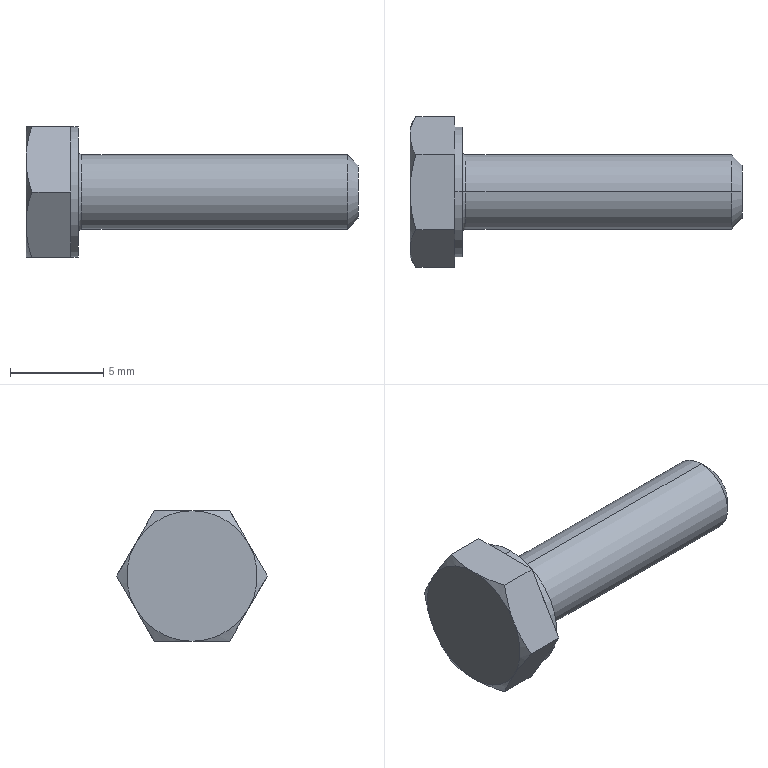Part | SolidWorks | features RevCut 4, Chamfer 1, Extrusion 1, Fillet 1, LPattern 1, Revolution 1 | 1 solid | 29 faces | box 17.8 x 8.083 x 7 mm | volume 303.684 mm3 | plane 15 | cone 8 | cylinder 4 | torus 2 | commonest cylinder face diameters 4 x2 7 x2
STEP:
#1=CARTESIAN_POINT('',(3.,0.,2.));
#2=VERTEX_POINT('',#1);
#3=CARTESIAN_POINT('',(3.,0.,-2.));
#4=VERTEX_POINT('',#3);
#5=CARTESIAN_POINT('',(3.,0.,0.));
#6=DIRECTION('',(1.,0.,0.));
#7=DIRECTION('',(0.,0.,-1.));
#8=AXIS2_PLACEMENT_3D('',#5,#6,#7);
#9=CIRCLE('',#8,2.);
#10=EDGE_CURVE('',#2,#4,#9,.T.);
#11=ORIENTED_EDGE('',*,*,#10,.F.);
#12=CARTESIAN_POINT('',(2.8,0.,2.2));
#13=VERTEX_POINT('',#12);
#14=CARTESIAN_POINT('',(3.,0.,2.2));
#15=DIRECTION('',(0.,1.,0.));
#16=DIRECTION('',(0.,0.,1.));
#17=AXIS2_PLACEMENT_3D('',#14,#15,#16);
#18=CIRCLE('',#17,0.2);
#19=EDGE_CURVE('',#2,#13,#18,.T.);
#20=ORIENTED_EDGE('',*,*,#19,.T.);
#21=CARTESIAN_POINT('',(2.8,0.,-2.2));
#22=VERTEX_POINT('',#21);
#23=CARTESIAN_POINT('',(2.8,0.,0.));
#24=DIRECTION('',(-1.,0.,0.));
#25=DIRECTION('',(0.,0.,-1.));
#26=AXIS2_PLACEMENT_3D('',#23,#24,#25);
#27=CIRCLE('',#26,2.2);
#28=EDGE_CURVE('',#22,#13,#27,.T.);
#29=ORIENTED_EDGE('',*,*,#28,.F.);
#30=CARTESIAN_POINT('',(3.,0.,-2.2));
#31=DIRECTION('',(0.,-1.,0.));
#32=DIRECTION('',(0.,0.,-1.));
#33=AXIS2_PLACEMENT_3D('',#30,#31,#32);
#34=CIRCLE('',#33,0.2);
#35=EDGE_CURVE('',#4,#22,#34,.T.);
#36=ORIENTED_EDGE('',*,*,#35,.F.);
#37=EDGE_LOOP('',(#11,#20,#29,#36));
#38=FACE_OUTER_BOUND('',#37,.T.);
#39=CARTESIAN_POINT('',(3.,0.,0.));
#40=DIRECTION('',(1.,0.,0.));
#41=DIRECTION('',(0.,0.,-1.));
#42=AXIS2_PLACEMENT_3D('',#39,#40,#41);
#43=TOROIDAL_SURFACE('',#42,2.2,0.2);
#44=ADVANCED_FACE('',(#38),#43,.F.);
#45=CARTESIAN_POINT('',(17.8,0.,-1.44));
#46=VERTEX_POINT('',#45);
#47=CARTESIAN_POINT('',(17.8,0.,1.44));
#48=VERTEX_POINT('',#47);
#49=CARTESIAN_POINT('',(17.8,0.,0.));
#50=DIRECTION('',(1.,0.,0.));
#51=DIRECTION('',(0.,0.,1.));
#52=AXIS2_PLACEMENT_3D('',#49,#50,#51);
#53=CIRCLE('',#52,1.44);
#54=EDGE_CURVE('',#46,#48,#53,.T.);
#55=ORIENTED_EDGE('',*,*,#54,.F.);
#56=CARTESIAN_POINT('',(17.24,0.,-2.));
#57=VERTEX_POINT('',#56);
#58=CARTESIAN_POINT('',(17.24,0.,-2.));
#59=DIRECTION('',(-0.7071,0.,-0.7071));
#60=VECTOR('',#59,1000.);
#61=LINE('',#58,#60);
#62=EDGE_CURVE('',#46,#57,#61,.T.);
#63=ORIENTED_EDGE('',*,*,#62,.T.);
#64=CARTESIAN_POINT('',(17.24,0.,2.));
#65=VERTEX_POINT('',#64);
#66=CARTESIAN_POINT('',(17.24,0.,0.));
#67=DIRECTION('',(-1.,0.,0.));
#68=DIRECTION('',(0.,0.,1.));
#69=AXIS2_PLACEMENT_3D('',#66,#67,#68);
#70=CIRCLE('',#69,2.);
#71=EDGE_CURVE('',#65,#57,#70,.T.);
#72=ORIENTED_EDGE('',*,*,#71,.F.);
#73=CARTESIAN_POINT('',(17.24,0.,2.));
#74=DIRECTION('',(-0.7071,0.,0.7071));
#75=VECTOR('',#74,1000.);
#76=LINE('',#73,#75);
#77=EDGE_CURVE('',#48,#65,#76,.T.);
#78=ORIENTED_EDGE('',*,*,#77,.F.);
#79=EDGE_LOOP('',(#55,#63,#72,#78));
#80=FACE_OUTER_BOUND('',#79,.T.);
#81=CARTESIAN_POINT('',(17.24,0.,0.));
#82=DIRECTION('',(-1.,0.,0.));
#83=DIRECTION('',(0.,0.,1.));
#84=AXIS2_PLACEMENT_3D('',#81,#82,#83);
#85=CONICAL_SURFACE('',#84,2.,0.7854);
#86=ADVANCED_FACE('',(#80),#85,.T.);
#87=ORIENTED_EDGE('',*,*,#71,.T.);
#88=CARTESIAN_POINT('',(0.,0.,-2.));
#89=DIRECTION('',(-1.,0.,0.));
#90=VECTOR('',#89,1000.);
#91=LINE('',#88,#90);
#92=EDGE_CURVE('',#57,#4,#91,.T.);
#93=ORIENTED_EDGE('',*,*,#92,.T.);
#94=CARTESIAN_POINT('',(3.,0.,0.));
#95=DIRECTION('',(1.,0.,0.));
#96=DIRECTION('',(0.,0.,-1.));
#97=AXIS2_PLACEMENT_3D('',#94,#95,#96);
#98=CIRCLE('',#97,2.);
#99=EDGE_CURVE('',#4,#2,#98,.T.);
#100=ORIENTED_EDGE('',*,*,#99,.T.);
#101=CARTESIAN_POINT('',(0.,0.,2.));
#102=DIRECTION('',(-1.,0.,0.));
#103=VECTOR('',#102,1000.);
#104=LINE('',#101,#103);
#105=EDGE_CURVE('',#65,#2,#104,.T.);
#106=ORIENTED_EDGE('',*,*,#105,.F.);
#107=EDGE_LOOP('',(#87,#93,#100,#106));
#108=FACE_OUTER_BOUND('',#107,.T.);
#109=CARTESIAN_POINT('',(0.,0.,0.));
#110=DIRECTION('',(-1.,0.,0.));
#111=DIRECTION('',(0.,0.,1.));
#112=AXIS2_PLACEMENT_3D('',#109,#110,#111);
#113=CYLINDRICAL_SURFACE('',#112,2.);
#114=ADVANCED_FACE('',(#108),#113,.T.);
#115=CARTESIAN_POINT('',(2.8,0.,-3.5));
#116=VERTEX_POINT('',#115);
#117=CARTESIAN_POINT('',(2.8,0.,3.5));
#118=VERTEX_POINT('',#117);
#119=CARTESIAN_POINT('',(2.8,0.,0.));
#120=DIRECTION('',(1.,0.,0.));
#121=DIRECTION('',(0.,0.,-1.));
#122=AXIS2_PLACEMENT_3D('',#119,#120,#121);
#123=CIRCLE('',#122,3.5);
#124=EDGE_CURVE('',#116,#118,#123,.T.);
#125=ORIENTED_EDGE('',*,*,#124,.F.);
#126=CARTESIAN_POINT('',(2.4,0.,-3.5));
#127=VERTEX_POINT('',#126);
#128=CARTESIAN_POINT('',(0.,0.,-3.5));
#129=DIRECTION('',(-1.,0.,0.));
#130=VECTOR('',#129,1000.);
#131=LINE('',#128,#130);
#132=EDGE_CURVE('',#116,#127,#131,.T.);
#133=ORIENTED_EDGE('',*,*,#132,.T.);
#134=CARTESIAN_POINT('',(2.4,3.031,-1.75));
#135=VERTEX_POINT('',#134);
#136=CARTESIAN_POINT('',(2.4,0.,0.));
#137=DIRECTION('',(-1.,0.,0.));
#138=DIRECTION('',(0.,0.,1.));
#139=AXIS2_PLACEMENT_3D('',#136,#137,#138);
#140=CIRCLE('',#139,3.5);
#141=EDGE_CURVE('',#135,#127,#140,.T.);
#142=ORIENTED_EDGE('',*,*,#141,.F.);
#143=CARTESIAN_POINT('',(2.4,3.031,1.75));
#144=VERTEX_POINT('',#143);
#145=CARTESIAN_POINT('',(2.4,0.,0.));
#146=DIRECTION('',(-1.,0.,0.));
#147=DIRECTION('',(0.,0.,1.));
#148=AXIS2_PLACEMENT_3D('',#145,#146,#147);
#149=CIRCLE('',#148,3.5);
#150=EDGE_CURVE('',#144,#135,#149,.T.);
#151=ORIENTED_EDGE('',*,*,#150,.F.);
#152=CARTESIAN_POINT('',(2.4,0.,3.5));
#153=VERTEX_POINT('',#152);
#154=CARTESIAN_POINT('',(2.4,0.,0.));
#155=DIRECTION('',(-1.,0.,0.));
#156=DIRECTION('',(0.,0.,1.));
#157=AXIS2_PLACEMENT_3D('',#154,#155,#156);
#158=CIRCLE('',#157,3.5);
#159=EDGE_CURVE('',#153,#144,#158,.T.);
#160=ORIENTED_EDGE('',*,*,#159,.F.);
#161=CARTESIAN_POINT('',(0.,0.,3.5));
#162=DIRECTION('',(-1.,0.,0.));
#163=VECTOR('',#162,1000.);
#164=LINE('',#161,#163);
#165=EDGE_CURVE('',#118,#153,#164,.T.);
#166=ORIENTED_EDGE('',*,*,#165,.F.);
#167=EDGE_LOOP('',(#125,#133,#142,#151,#160,#166));
#168=FACE_OUTER_BOUND('',#167,.T.);
#169=CARTESIAN_POINT('',(0.,0.,0.));
#170=DIRECTION('',(-1.,0.,0.));
#171=DIRECTION('',(0.,0.,1.));
#172=AXIS2_PLACEMENT_3D('',#169,#170,#171);
#173=CYLINDRICAL_SURFACE('',#172,3.5);
#174=ADVANCED_FACE('',(#168),#173,.T.);
#175=CARTESIAN_POINT('',(2.4,2.021,-3.5));
#176=VERTEX_POINT('',#175);
#177=CARTESIAN_POINT('',(2.4,2.021,-3.5));
#178=DIRECTION('',(0.,0.5,0.866));
#179=VECTOR('',#178,1000.);
#180=LINE('',#177,#179);
#181=EDGE_CURVE('',#176,#135,#180,.T.);
#182=ORIENTED_EDGE('',*,*,#181,.F.);
#183=CARTESIAN_POINT('',(0.3126,2.021,-3.5));
#184=VERTEX_POINT('',#183);
#185=CARTESIAN_POINT('',(2.8,2.021,-3.5));
#186=DIRECTION('',(-1.,0.,0.));
#187=VECTOR('',#186,1000.);
#188=LINE('',#185,#187);
#189=EDGE_CURVE('',#176,#184,#188,.T.);
#190=ORIENTED_EDGE('',*,*,#189,.T.);
#191=CARTESIAN_POINT('',(0.,3.031,-1.75));
#192=VERTEX_POINT('',#191);
#193=CARTESIAN_POINT('',(0.,3.031,-1.75));
#194=CARTESIAN_POINT('',(0.,2.86,-2.047));
#195=CARTESIAN_POINT('',(0.02993,2.688,-2.344));
#196=CARTESIAN_POINT('',(0.1388,2.352,-2.926));
#197=CARTESIAN_POINT('',(0.2174,2.186,-3.214));
#198=CARTESIAN_POINT('',(0.3126,2.021,-3.5));
#199=B_SPLINE_CURVE_WITH_KNOTS('',3,(#193,#194,#195,#196,#197,#198),.UNSPECIFIED.,.F.,.F.,(4,2,4),(0.002045,0.003063,0.004082),.UNSPECIFIED.);
#200=EDGE_CURVE('',#192,#184,#199,.T.);
#201=ORIENTED_EDGE('',*,*,#200,.F.);
#202=CARTESIAN_POINT('',(0.3126,4.041,0.));
#203=VERTEX_POINT('',#202);
#204=CARTESIAN_POINT('',(0.3126,4.041,0.));
#205=CARTESIAN_POINT('',(0.1218,3.711,-0.5726));
#206=CARTESIAN_POINT('',(0.,3.375,-1.154));
#207=CARTESIAN_POINT('',(0.,3.031,-1.75));
#208=B_SPLINE_CURVE_WITH_KNOTS('',3,(#204,#205,#206,#207),.UNSPECIFIED.,.F.,.F.,(4,4),(0.000000238,0.002045),.UNSPECIFIED.);
#209=EDGE_CURVE('',#203,#192,#208,.T.);
#210=ORIENTED_EDGE('',*,*,#209,.F.);
#211=CARTESIAN_POINT('',(2.4,4.041,0.));
#212=VERTEX_POINT('',#211);
#213=CARTESIAN_POINT('',(2.8,4.041,0.));
#214=DIRECTION('',(-1.,0.,0.));
#215=VECTOR('',#214,1000.);
#216=LINE('',#213,#215);
#217=EDGE_CURVE('',#212,#203,#216,.T.);
#218=ORIENTED_EDGE('',*,*,#217,.F.);
#219=CARTESIAN_POINT('',(2.4,2.021,-3.5));
#220=DIRECTION('',(0.,0.5,0.866));
#221=VECTOR('',#220,1000.);
#222=LINE('',#219,#221);
#223=EDGE_CURVE('',#135,#212,#222,.T.);
#224=ORIENTED_EDGE('',*,*,#223,.F.);
#225=EDGE_LOOP('',(#182,#190,#201,#210,#218,#224));
#226=FACE_OUTER_BOUND('',#225,.T.);
#227=CARTESIAN_POINT('',(2.8,2.021,-3.5));
#228=DIRECTION('',(0.,-0.866,0.5));
#229=DIRECTION('',(0.,-0.5,-0.866));
#230=AXIS2_PLACEMENT_3D('',#227,#228,#229);
#231=PLANE('',#230);
#232=ADVANCED_FACE('',(#226),#231,.F.);
#233=CARTESIAN_POINT('',(2.4,4.041,0.));
#234=DIRECTION('',(0.,-0.5,0.866));
#235=VECTOR('',#234,1000.);
#236=LINE('',#233,#235);
#237=EDGE_CURVE('',#212,#144,#236,.T.);
#238=ORIENTED_EDGE('',*,*,#237,.F.);
#239=ORIENTED_EDGE('',*,*,#217,.T.);
#240=CARTESIAN_POINT('',(0.,3.031,1.75));
#241=VERTEX_POINT('',#240);
#242=CARTESIAN_POINT('',(0.,3.031,1.75));
#243=CARTESIAN_POINT('',(0.,3.203,1.453));
#244=CARTESIAN_POINT('',(0.02993,3.374,1.156));
#245=CARTESIAN_POINT('',(0.1388,3.71,0.5735));
#246=CARTESIAN_POINT('',(0.2174,3.877,0.2856));
#247=CARTESIAN_POINT('',(0.3126,4.041,0.));
#248=B_SPLINE_CURVE_WITH_KNOTS('',3,(#242,#243,#244,#245,#246,#247),.UNSPECIFIED.,.F.,.F.,(4,2,4),(0.002045,0.003063,0.004082),.UNSPECIFIED.);
#249=EDGE_CURVE('',#241,#203,#248,.T.);
#250=ORIENTED_EDGE('',*,*,#249,.F.);
#251=CARTESIAN_POINT('',(0.3126,2.021,3.5));
#252=VERTEX_POINT('',#251);
#253=CARTESIAN_POINT('',(0.3126,2.021,3.5));
#254=CARTESIAN_POINT('',(0.1218,2.351,2.927));
#255=CARTESIAN_POINT('',(0.,2.687,2.346));
#256=CARTESIAN_POINT('',(0.,3.031,1.75));
#257=B_SPLINE_CURVE_WITH_KNOTS('',3,(#253,#254,#255,#256),.UNSPECIFIED.,.F.,.F.,(4,4),(0.000000238,0.002045),.UNSPECIFIED.);
#258=EDGE_CURVE('',#252,#241,#257,.T.);
#259=ORIENTED_EDGE('',*,*,#258,.F.);
#260=CARTESIAN_POINT('',(2.4,2.021,3.5));
#261=VERTEX_POINT('',#260);
#262=CARTESIAN_POINT('',(2.8,2.021,3.5));
#263=DIRECTION('',(-1.,0.,0.));
#264=VECTOR('',#263,1000.);
#265=LINE('',#262,#264);
#266=EDGE_CURVE('',#261,#252,#265,.T.);
#267=ORIENTED_EDGE('',*,*,#266,.F.);
#268=CARTESIAN_POINT('',(2.4,4.041,0.));
#269=DIRECTION('',(0.,-0.5,0.866));
#270=VECTOR('',#269,1000.);
#271=LINE('',#268,#270);
#272=EDGE_CURVE('',#144,#261,#271,.T.);
#273=ORIENTED_EDGE('',*,*,#272,.F.);
#274=EDGE_LOOP('',(#238,#239,#250,#259,#267,#273));
#275=FACE_OUTER_BOUND('',#274,.T.);
#276=CARTESIAN_POINT('',(2.8,4.041,0.));
#277=DIRECTION('',(0.,-0.866,-0.5));
#278=DIRECTION('',(0.,0.5,-0.866));
#279=AXIS2_PLACEMENT_3D('',#276,#277,#278);
#280=PLANE('',#279);
#281=ADVANCED_FACE('',(#275),#280,.F.);
#282=CARTESIAN_POINT('',(2.4,2.021,3.5));
#283=DIRECTION('',(0.,-1.,0.));
#284=VECTOR('',#283,1000.);
#285=LINE('',#282,#284);
#286=EDGE_CURVE('',#261,#153,#285,.T.);
#287=ORIENTED_EDGE('',*,*,#286,.F.);
#288=ORIENTED_EDGE('',*,*,#266,.T.);
#289=CARTESIAN_POINT('',(0.,0.,3.5));
#290=VERTEX_POINT('',#289);
#291=CARTESIAN_POINT('',(0.,0.,3.5));
#292=CARTESIAN_POINT('',(0.,0.3423,3.5));
#293=CARTESIAN_POINT('',(0.03026,0.6887,3.5));
#294=CARTESIAN_POINT('',(0.1397,1.363,3.5));
#295=CARTESIAN_POINT('',(0.2182,1.694,3.5));
#296=CARTESIAN_POINT('',(0.3126,2.021,3.5));
#297=B_SPLINE_CURVE_WITH_KNOTS('',3,(#291,#292,#293,#294,#295,#296),.UNSPECIFIED.,.F.,.F.,(4,2,4),(0.00582,0.006844,0.007868),.UNSPECIFIED.);
#298=EDGE_CURVE('',#290,#252,#297,.T.);
#299=ORIENTED_EDGE('',*,*,#298,.F.);
#300=CARTESIAN_POINT('',(0.3126,-2.021,3.5));
#301=VERTEX_POINT('',#300);
#302=CARTESIAN_POINT('',(0.3126,-2.021,3.5));
#303=CARTESIAN_POINT('',(0.2176,-1.692,3.5));
#304=CARTESIAN_POINT('',(0.1381,-1.355,3.5));
#305=CARTESIAN_POINT('',(0.02943,-0.6813,3.5));
#306=CARTESIAN_POINT('',(0.,-0.342,3.5));
#307=CARTESIAN_POINT('',(0.,0.,3.5));
#308=B_SPLINE_CURVE_WITH_KNOTS('',3,(#302,#303,#304,#305,#306,#307),.UNSPECIFIED.,.F.,.F.,(4,2,4),(0.003774,0.004797,0.00582),.UNSPECIFIED.);
#309=EDGE_CURVE('',#301,#290,#308,.T.);
#310=ORIENTED_EDGE('',*,*,#309,.F.);
#311=CARTESIAN_POINT('',(2.4,-2.021,3.5));
#312=VERTEX_POINT('',#311);
#313=CARTESIAN_POINT('',(2.8,-2.021,3.5));
#314=DIRECTION('',(-1.,0.,0.));
#315=VECTOR('',#314,1000.);
#316=LINE('',#313,#315);
#317=EDGE_CURVE('',#312,#301,#316,.T.);
#318=ORIENTED_EDGE('',*,*,#317,.F.);
#319=CARTESIAN_POINT('',(2.4,2.021,3.5));
#320=DIRECTION('',(0.,-1.,0.));
#321=VECTOR('',#320,1000.);
#322=LINE('',#319,#321);
#323=EDGE_CURVE('',#153,#312,#322,.T.);
#324=ORIENTED_EDGE('',*,*,#323,.F.);
#325=EDGE_LOOP('',(#287,#288,#299,#310,#318,#324));
#326=FACE_OUTER_BOUND('',#325,.T.);
#327=CARTESIAN_POINT('',(2.8,2.021,3.5));
#328=DIRECTION('',(0.,0.,-1.));
#329=DIRECTION('',(0.,1.,0.));
#330=AXIS2_PLACEMENT_3D('',#327,#328,#329);
#331=PLANE('',#330);
#332=ADVANCED_FACE('',(#326),#331,.F.);
#333=CARTESIAN_POINT('',(2.4,-3.031,1.75));
#334=VERTEX_POINT('',#333);
#335=CARTESIAN_POINT('',(2.4,-4.041,0.));
#336=DIRECTION('',(0.,-0.5,-0.866));
#337=VECTOR('',#336,1000.);
#338=LINE('',#335,#337);
#339=EDGE_CURVE('',#312,#334,#338,.T.);
#340=ORIENTED_EDGE('',*,*,#339,.F.);
#341=ORIENTED_EDGE('',*,*,#317,.T.);
#342=CARTESIAN_POINT('',(0.,-3.031,1.75));
#343=VERTEX_POINT('',#342);
#344=CARTESIAN_POINT('',(0.,-3.031,1.75));
#345=CARTESIAN_POINT('',(0.,-2.86,2.047));
#346=CARTESIAN_POINT('',(0.02993,-2.688,2.344));
#347=CARTESIAN_POINT('',(0.1388,-2.352,2.926));
#348=CARTESIAN_POINT('',(0.2174,-2.186,3.214));
#349=CARTESIAN_POINT('',(0.3126,-2.021,3.5));
#350=B_SPLINE_CURVE_WITH_KNOTS('',3,(#344,#345,#346,#347,#348,#349),.UNSPECIFIED.,.F.,.F.,(4,2,4),(0.002045,0.003063,0.004082),.UNSPECIFIED.);
#351=EDGE_CURVE('',#343,#301,#350,.T.);
#352=ORIENTED_EDGE('',*,*,#351,.F.);
#353=CARTESIAN_POINT('',(0.3126,-4.041,0.));
#354=VERTEX_POINT('',#353);
#355=CARTESIAN_POINT('',(0.3126,-4.041,0.));
#356=CARTESIAN_POINT('',(0.1218,-3.711,0.5726));
#357=CARTESIAN_POINT('',(0.,-3.375,1.154));
#358=CARTESIAN_POINT('',(0.,-3.031,1.75));
#359=B_SPLINE_CURVE_WITH_KNOTS('',3,(#355,#356,#357,#358),.UNSPECIFIED.,.F.,.F.,(4,4),(0.000000238,0.002045),.UNSPECIFIED.);
#360=EDGE_CURVE('',#354,#343,#359,.T.);
#361=ORIENTED_EDGE('',*,*,#360,.F.);
#362=CARTESIAN_POINT('',(2.4,-4.041,0.));
#363=VERTEX_POINT('',#362);
#364=CARTESIAN_POINT('',(2.8,-4.041,0.));
#365=DIRECTION('',(-1.,0.,0.));
#366=VECTOR('',#365,1000.);
#367=LINE('',#364,#366);
#368=EDGE_CURVE('',#363,#354,#367,.T.);
#369=ORIENTED_EDGE('',*,*,#368,.F.);
#370=CARTESIAN_POINT('',(2.4,-4.041,0.));
#371=DIRECTION('',(0.,-0.5,-0.866));
#372=VECTOR('',#371,1000.);
#373=LINE('',#370,#372);
#374=EDGE_CURVE('',#334,#363,#373,.T.);
#375=ORIENTED_EDGE('',*,*,#374,.F.);
#376=EDGE_LOOP('',(#340,#341,#352,#361,#369,#375));
#377=FACE_OUTER_BOUND('',#376,.T.);
#378=CARTESIAN_POINT('',(2.8,-4.041,0.));
#379=DIRECTION('',(0.,0.866,-0.5));
#380=DIRECTION('',(0.,0.5,0.866));
#381=AXIS2_PLACEMENT_3D('',#378,#379,#380);
#382=PLANE('',#381);
#383=ADVANCED_FACE('',(#377),#382,.F.);
#384=CARTESIAN_POINT('',(2.4,-3.031,-1.75));
#385=VERTEX_POINT('',#384);
#386=CARTESIAN_POINT('',(2.4,-2.021,-3.5));
#387=DIRECTION('',(0.,0.5,-0.866));
#388=VECTOR('',#387,1000.);
#389=LINE('',#386,#388);
#390=EDGE_CURVE('',#363,#385,#389,.T.);
#391=ORIENTED_EDGE('',*,*,#390,.F.);
#392=ORIENTED_EDGE('',*,*,#368,.T.);
#393=CARTESIAN_POINT('',(0.,-3.031,-1.75));
#394=VERTEX_POINT('',#393);
#395=CARTESIAN_POINT('',(0.,-3.031,-1.75));
#396=CARTESIAN_POINT('',(0.,-3.203,-1.453));
#397=CARTESIAN_POINT('',(0.02993,-3.374,-1.156));
#398=CARTESIAN_POINT('',(0.1388,-3.71,-0.5735));
#399=CARTESIAN_POINT('',(0.2174,-3.877,-0.2856));
#400=CARTESIAN_POINT('',(0.3126,-4.041,0.));
#401=B_SPLINE_CURVE_WITH_KNOTS('',3,(#395,#396,#397,#398,#399,#400),.UNSPECIFIED.,.F.,.F.,(4,2,4),(0.002045,0.003063,0.004082),.UNSPECIFIED.);
#402=EDGE_CURVE('',#394,#354,#401,.T.);
#403=ORIENTED_EDGE('',*,*,#402,.F.);
#404=CARTESIAN_POINT('',(0.3126,-2.021,-3.5));
#405=VERTEX_POINT('',#404);
#406=CARTESIAN_POINT('',(0.3126,-2.021,-3.5));
#407=CARTESIAN_POINT('',(0.1218,-2.351,-2.927));
#408=CARTESIAN_POINT('',(0.,-2.687,-2.346));
#409=CARTESIAN_POINT('',(0.,-3.031,-1.75));
#410=B_SPLINE_CURVE_WITH_KNOTS('',3,(#406,#407,#408,#409),.UNSPECIFIED.,.F.,.F.,(4,4),(0.000000238,0.002045),.UNSPECIFIED.);
#411=EDGE_CURVE('',#405,#394,#410,.T.);
#412=ORIENTED_EDGE('',*,*,#411,.F.);
#413=CARTESIAN_POINT('',(2.4,-2.021,-3.5));
#414=VERTEX_POINT('',#413);
#415=CARTESIAN_POINT('',(2.8,-2.021,-3.5));
#416=DIRECTION('',(-1.,0.,0.));
#417=VECTOR('',#416,1000.);
#418=LINE('',#415,#417);
#419=EDGE_CURVE('',#414,#405,#418,.T.);
#420=ORIENTED_EDGE('',*,*,#419,.F.);
#421=CARTESIAN_POINT('',(2.4,-2.021,-3.5));
#422=DIRECTION('',(0.,0.5,-0.866));
#423=VECTOR('',#422,1000.);
#424=LINE('',#421,#423);
#425=EDGE_CURVE('',#385,#414,#424,.T.);
#426=ORIENTED_EDGE('',*,*,#425,.F.);
#427=EDGE_LOOP('',(#391,#392,#403,#412,#420,#426));
#428=FACE_OUTER_BOUND('',#427,.T.);
#429=CARTESIAN_POINT('',(2.8,-2.021,-3.5));
#430=DIRECTION('',(0.,0.866,0.5));
#431=DIRECTION('',(0.,-0.5,0.866));
#432=AXIS2_PLACEMENT_3D('',#429,#430,#431);
#433=PLANE('',#432);
#434=ADVANCED_FACE('',(#428),#433,.F.);
#435=CARTESIAN_POINT('',(2.4,2.021,-3.5));
#436=DIRECTION('',(0.,1.,0.));
#437=VECTOR('',#436,1000.);
#438=LINE('',#435,#437);
#439=EDGE_CURVE('',#414,#127,#438,.T.);
#440=ORIENTED_EDGE('',*,*,#439,.F.);
#441=ORIENTED_EDGE('',*,*,#419,.T.);
#442=CARTESIAN_POINT('',(0.,0.,-3.5));
#443=VERTEX_POINT('',#442);
#444=CARTESIAN_POINT('',(0.,0.,-3.5));
#445=CARTESIAN_POINT('',(0.,-0.342,-3.5));
#446=CARTESIAN_POINT('',(0.02943,-0.6813,-3.5));
#447=CARTESIAN_POINT('',(0.1381,-1.355,-3.5));
#448=CARTESIAN_POINT('',(0.2176,-1.692,-3.5));
#449=CARTESIAN_POINT('',(0.3126,-2.021,-3.5));
#450=B_SPLINE_CURVE_WITH_KNOTS('',3,(#444,#445,#446,#447,#448,#449),.UNSPECIFIED.,.F.,.F.,(4,2,4),(0.01285,0.01387,0.0149),.UNSPECIFIED.);
#451=EDGE_CURVE('',#443,#405,#450,.T.);
#452=ORIENTED_EDGE('',*,*,#451,.F.);
#453=CARTESIAN_POINT('',(0.3126,2.021,-3.5));
#454=CARTESIAN_POINT('',(0.2182,1.694,-3.5));
#455=CARTESIAN_POINT('',(0.1397,1.363,-3.5));
#456=CARTESIAN_POINT('',(0.03026,0.6887,-3.5));
#457=CARTESIAN_POINT('',(0.,0.3423,-3.5));
#458=CARTESIAN_POINT('',(0.,0.,-3.5));
#459=B_SPLINE_CURVE_WITH_KNOTS('',3,(#453,#454,#455,#456,#457,#458),.UNSPECIFIED.,.F.,.F.,(4,2,4),(0.01081,0.01183,0.01285),.UNSPECIFIED.);
#460=EDGE_CURVE('',#184,#443,#459,.T.);
#461=ORIENTED_EDGE('',*,*,#460,.F.);
#462=ORIENTED_EDGE('',*,*,#189,.F.);
#463=CARTESIAN_POINT('',(2.4,2.021,-3.5));
#464=DIRECTION('',(0.,1.,0.));
#465=VECTOR('',#464,1000.);
#466=LINE('',#463,#465);
#467=EDGE_CURVE('',#127,#176,#466,.T.);
#468=ORIENTED_EDGE('',*,*,#467,.F.);
#469=EDGE_LOOP('',(#440,#441,#452,#461,#462,#468));
#470=FACE_OUTER_BOUND('',#469,.T.);
#471=CARTESIAN_POINT('',(2.8,2.021,-3.5));
#472=DIRECTION('',(0.,0.,1.));
#473=DIRECTION('',(0.,-1.,0.));
#474=AXIS2_PLACEMENT_3D('',#471,#472,#473);
#475=PLANE('',#474);
#476=ADVANCED_FACE('',(#470),#475,.F.);
#477=ORIENTED_EDGE('',*,*,#411,.T.);
#478=CARTESIAN_POINT('',(0.,0.,0.));
#479=DIRECTION('',(1.,0.,0.));
#480=DIRECTION('',(0.,0.,-1.));
#481=AXIS2_PLACEMENT_3D('',#478,#479,#480);
#482=CIRCLE('',#481,3.5);
#483=EDGE_CURVE('',#394,#443,#482,.T.);
#484=ORIENTED_EDGE('',*,*,#483,.T.);
#485=ORIENTED_EDGE('',*,*,#451,.T.);
#486=EDGE_LOOP('',(#477,#484,#485));
#487=FACE_OUTER_BOUND('',#486,.T.);
#488=CARTESIAN_POINT('',(0.,0.,0.));
#489=DIRECTION('',(1.,0.,0.));
#490=DIRECTION('',(0.,0.,-1.));
#491=AXIS2_PLACEMENT_3D('',#488,#489,#490);
#492=CONICAL_SURFACE('',#491,3.5,1.047);
#493=ADVANCED_FACE('',(#487),#492,.T.);
#494=ORIENTED_EDGE('',*,*,#360,.T.);
#495=CARTESIAN_POINT('',(0.,0.,0.));
#496=DIRECTION('',(1.,0.,0.));
#497=DIRECTION('',(0.,0.,-1.));
#498=AXIS2_PLACEMENT_3D('',#495,#496,#497);
#499=CIRCLE('',#498,3.5);
#500=EDGE_CURVE('',#343,#394,#499,.T.);
#501=ORIENTED_EDGE('',*,*,#500,.T.);
#502=ORIENTED_EDGE('',*,*,#402,.T.);
#503=EDGE_LOOP('',(#494,#501,#502));
#504=FACE_OUTER_BOUND('',#503,.T.);
#505=CARTESIAN_POINT('',(0.,0.,0.));
#506=DIRECTION('',(1.,0.,0.));
#507=DIRECTION('',(0.,0.,-1.));
#508=AXIS2_PLACEMENT_3D('',#505,#506,#507);
#509=CONICAL_SURFACE('',#508,3.5,1.047);
#510=ADVANCED_FACE('',(#504),#509,.T.);
#511=ORIENTED_EDGE('',*,*,#309,.T.);
#512=CARTESIAN_POINT('',(0.,0.,0.));
#513=DIRECTION('',(1.,0.,0.));
#514=DIRECTION('',(0.,0.,-1.));
#515=AXIS2_PLACEMENT_3D('',#512,#513,#514);
#516=CIRCLE('',#515,3.5);
#517=EDGE_CURVE('',#290,#343,#516,.T.);
#518=ORIENTED_EDGE('',*,*,#517,.T.);
#519=ORIENTED_EDGE('',*,*,#351,.T.);
#520=EDGE_LOOP('',(#511,#518,#519));
#521=FACE_OUTER_BOUND('',#520,.T.);
#522=CARTESIAN_POINT('',(0.,0.,0.));
#523=DIRECTION('',(1.,0.,0.));
#524=DIRECTION('',(0.,0.,-1.));
#525=AXIS2_PLACEMENT_3D('',#522,#523,#524);
#526=CONICAL_SURFACE('',#525,3.5,1.047);
#527=ADVANCED_FACE('',(#521),#526,.T.);
#528=ORIENTED_EDGE('',*,*,#298,.T.);
#529=ORIENTED_EDGE('',*,*,#258,.T.);
#530=CARTESIAN_POINT('',(0.,0.,0.));
#531=DIRECTION('',(-1.,0.,0.));
#532=DIRECTION('',(0.,0.,1.));
#533=AXIS2_PLACEMENT_3D('',#530,#531,#532);
#534=CIRCLE('',#533,3.5);
#535=EDGE_CURVE('',#290,#241,#534,.T.);
#536=ORIENTED_EDGE('',*,*,#535,.F.);
#537=EDGE_LOOP('',(#528,#529,#536));
#538=FACE_OUTER_BOUND('',#537,.T.);
#539=CARTESIAN_POINT('',(0.,0.,0.));
#540=DIRECTION('',(1.,0.,0.));
#541=DIRECTION('',(0.,0.,-1.));
#542=AXIS2_PLACEMENT_3D('',#539,#540,#541);
#543=CONICAL_SURFACE('',#542,3.5,1.047);
#544=ADVANCED_FACE('',(#538),#543,.T.);
#545=ORIENTED_EDGE('',*,*,#249,.T.);
#546=ORIENTED_EDGE('',*,*,#209,.T.);
#547=CARTESIAN_POINT('',(0.,0.,0.));
#548=DIRECTION('',(1.,0.,0.));
#549=DIRECTION('',(0.,0.,-1.));
#550=AXIS2_PLACEMENT_3D('',#547,#548,#549);
#551=CIRCLE('',#550,3.5);
#552=EDGE_CURVE('',#192,#241,#551,.T.);
#553=ORIENTED_EDGE('',*,*,#552,.T.);
#554=EDGE_LOOP('',(#545,#546,#553));
#555=FACE_OUTER_BOUND('',#554,.T.);
#556=CARTESIAN_POINT('',(0.,0.,0.));
#557=DIRECTION('',(1.,0.,0.));
#558=DIRECTION('',(0.,0.,-1.));
#559=AXIS2_PLACEMENT_3D('',#556,#557,#558);
#560=CONICAL_SURFACE('',#559,3.5,1.047);
#561=ADVANCED_FACE('',(#555),#560,.T.);
#562=ORIENTED_EDGE('',*,*,#200,.T.);
#563=ORIENTED_EDGE('',*,*,#460,.T.);
#564=CARTESIAN_POINT('',(0.,0.,0.));
#565=DIRECTION('',(1.,0.,0.));
#566=DIRECTION('',(0.,0.,-1.));
#567=AXIS2_PLACEMENT_3D('',#564,#565,#566);
#568=CIRCLE('',#567,3.5);
#569=EDGE_CURVE('',#443,#192,#568,.T.);
#570=ORIENTED_EDGE('',*,*,#569,.T.);
#571=EDGE_LOOP('',(#562,#563,#570));
#572=FACE_OUTER_BOUND('',#571,.T.);
#573=CARTESIAN_POINT('',(0.,0.,0.));
#574=DIRECTION('',(1.,0.,0.));
#575=DIRECTION('',(0.,0.,-1.));
#576=AXIS2_PLACEMENT_3D('',#573,#574,#575);
#577=CONICAL_SURFACE('',#576,3.5,1.047);
#578=ADVANCED_FACE('',(#572),#577,.T.);
#579=ORIENTED_EDGE('',*,*,#569,.F.);
#580=ORIENTED_EDGE('',*,*,#483,.F.);
#581=ORIENTED_EDGE('',*,*,#500,.F.);
#582=ORIENTED_EDGE('',*,*,#517,.F.);
#583=ORIENTED_EDGE('',*,*,#535,.T.);
#584=ORIENTED_EDGE('',*,*,#552,.F.);
#585=EDGE_LOOP('',(#579,#580,#581,#582,#583,#584));
#586=FACE_OUTER_BOUND('',#585,.T.);
#587=CARTESIAN_POINT('',(0.,0.,-7.));
#588=DIRECTION('',(1.,0.,0.));
#589=DIRECTION('',(0.,0.,-1.));
#590=AXIS2_PLACEMENT_3D('',#587,#588,#589);
#591=PLANE('',#590);
#592=ADVANCED_FACE('',(#586),#591,.F.);
#593=ORIENTED_EDGE('',*,*,#181,.T.);
#594=ORIENTED_EDGE('',*,*,#141,.T.);
#595=ORIENTED_EDGE('',*,*,#467,.T.);
#596=EDGE_LOOP('',(#593,#594,#595));
#597=FACE_OUTER_BOUND('',#596,.T.);
#598=CARTESIAN_POINT('',(2.4,3.5,0.));
#599=DIRECTION('',(1.,0.,0.));
#600=DIRECTION('',(0.,0.,-1.));
#601=AXIS2_PLACEMENT_3D('',#598,#599,#600);
#602=PLANE('',#601);
#603=ADVANCED_FACE('',(#597),#602,.T.);
#604=ORIENTED_EDGE('',*,*,#223,.T.);
#605=ORIENTED_EDGE('',*,*,#237,.T.);
#606=ORIENTED_EDGE('',*,*,#150,.T.);
#607=EDGE_LOOP('',(#604,#605,#606));
#608=FACE_OUTER_BOUND('',#607,.T.);
#609=CARTESIAN_POINT('',(2.4,3.5,0.));
#610=DIRECTION('',(1.,0.,0.));
#611=DIRECTION('',(0.,0.,-1.));
#612=AXIS2_PLACEMENT_3D('',#609,#610,#611);
#613=PLANE('',#612);
#614=ADVANCED_FACE('',(#608),#613,.T.);
#615=ORIENTED_EDGE('',*,*,#272,.T.);
#616=ORIENTED_EDGE('',*,*,#286,.T.);
#617=ORIENTED_EDGE('',*,*,#159,.T.);
#618=EDGE_LOOP('',(#615,#616,#617));
#619=FACE_OUTER_BOUND('',#618,.T.);
#620=CARTESIAN_POINT('',(2.4,3.5,0.));
#621=DIRECTION('',(1.,0.,0.));
#622=DIRECTION('',(0.,0.,-1.));
#623=AXIS2_PLACEMENT_3D('',#620,#621,#622);
#624=PLANE('',#623);
#625=ADVANCED_FACE('',(#619),#624,.T.);
#626=ORIENTED_EDGE('',*,*,#323,.T.);
#627=ORIENTED_EDGE('',*,*,#339,.T.);
#628=CARTESIAN_POINT('',(2.4,0.,0.));
#629=DIRECTION('',(-1.,0.,0.));
#630=DIRECTION('',(0.,0.,1.));
#631=AXIS2_PLACEMENT_3D('',#628,#629,#630);
#632=CIRCLE('',#631,3.5);
#633=EDGE_CURVE('',#334,#153,#632,.T.);
#634=ORIENTED_EDGE('',*,*,#633,.T.);
#635=EDGE_LOOP('',(#626,#627,#634));
#636=FACE_OUTER_BOUND('',#635,.T.);
#637=CARTESIAN_POINT('',(2.4,3.5,0.));
#638=DIRECTION('',(1.,0.,0.));
#639=DIRECTION('',(0.,0.,-1.));
#640=AXIS2_PLACEMENT_3D('',#637,#638,#639);
#641=PLANE('',#640);
#642=ADVANCED_FACE('',(#636),#641,.T.);
#643=ORIENTED_EDGE('',*,*,#374,.T.);
#644=ORIENTED_EDGE('',*,*,#390,.T.);
#645=CARTESIAN_POINT('',(2.4,0.,0.));
#646=DIRECTION('',(-1.,0.,0.));
#647=DIRECTION('',(0.,0.,1.));
#648=AXIS2_PLACEMENT_3D('',#645,#646,#647);
#649=CIRCLE('',#648,3.5);
#650=EDGE_CURVE('',#385,#334,#649,.T.);
#651=ORIENTED_EDGE('',*,*,#650,.T.);
#652=EDGE_LOOP('',(#643,#644,#651));
#653=FACE_OUTER_BOUND('',#652,.T.);
#654=CARTESIAN_POINT('',(2.4,3.5,0.));
#655=DIRECTION('',(1.,0.,0.));
#656=DIRECTION('',(0.,0.,-1.));
#657=AXIS2_PLACEMENT_3D('',#654,#655,#656);
#658=PLANE('',#657);
#659=ADVANCED_FACE('',(#653),#658,.T.);
#660=ORIENTED_EDGE('',*,*,#425,.T.);
#661=ORIENTED_EDGE('',*,*,#439,.T.);
#662=CARTESIAN_POINT('',(2.4,0.,0.));
#663=DIRECTION('',(-1.,0.,0.));
#664=DIRECTION('',(0.,0.,1.));
#665=AXIS2_PLACEMENT_3D('',#662,#663,#664);
#666=CIRCLE('',#665,3.5);
#667=EDGE_CURVE('',#127,#385,#666,.T.);
#668=ORIENTED_EDGE('',*,*,#667,.T.);
#669=EDGE_LOOP('',(#660,#661,#668));
#670=FACE_OUTER_BOUND('',#669,.T.);
#671=CARTESIAN_POINT('',(2.4,3.5,0.));
#672=DIRECTION('',(1.,0.,0.));
#673=DIRECTION('',(0.,0.,-1.));
#674=AXIS2_PLACEMENT_3D('',#671,#672,#673);
#675=PLANE('',#674);
#676=ADVANCED_FACE('',(#670),#675,.T.);
#677=ORIENTED_EDGE('',*,*,#132,.F.);
#678=CARTESIAN_POINT('',(2.8,0.,0.));
#679=DIRECTION('',(1.,0.,0.));
#680=DIRECTION('',(0.,0.,-1.));
#681=AXIS2_PLACEMENT_3D('',#678,#679,#680);
#682=CIRCLE('',#681,3.5);
#683=EDGE_CURVE('',#118,#116,#682,.T.);
#684=ORIENTED_EDGE('',*,*,#683,.F.);
#685=ORIENTED_EDGE('',*,*,#165,.T.);
#686=ORIENTED_EDGE('',*,*,#633,.F.);
#687=ORIENTED_EDGE('',*,*,#650,.F.);
#688=ORIENTED_EDGE('',*,*,#667,.F.);
#689=EDGE_LOOP('',(#677,#684,#685,#686,#687,#688));
#690=FACE_OUTER_BOUND('',#689,.T.);
#691=CARTESIAN_POINT('',(0.,0.,0.));
#692=DIRECTION('',(-1.,0.,0.));
#693=DIRECTION('',(0.,0.,1.));
#694=AXIS2_PLACEMENT_3D('',#691,#692,#693);
#695=CYLINDRICAL_SURFACE('',#694,3.5);
#696=ADVANCED_FACE('',(#690),#695,.T.);
#697=CARTESIAN_POINT('',(17.8,0.,0.));
#698=DIRECTION('',(1.,0.,0.));
#699=DIRECTION('',(0.,0.,1.));
#700=AXIS2_PLACEMENT_3D('',#697,#698,#699);
#701=CIRCLE('',#700,1.44);
#702=EDGE_CURVE('',#48,#46,#701,.T.);
#703=ORIENTED_EDGE('',*,*,#702,.T.);
#704=ORIENTED_EDGE('',*,*,#54,.T.);
#705=EDGE_LOOP('',(#703,#704));
#706=FACE_OUTER_BOUND('',#705,.T.);
#707=CARTESIAN_POINT('',(17.8,0.,0.));
#708=DIRECTION('',(-1.,0.,0.));
#709=DIRECTION('',(0.,0.,1.));
#710=AXIS2_PLACEMENT_3D('',#707,#708,#709);
#711=PLANE('',#710);
#712=ADVANCED_FACE('',(#706),#711,.F.);
#713=ORIENTED_EDGE('',*,*,#92,.F.);
#714=CARTESIAN_POINT('',(17.24,0.,0.));
#715=DIRECTION('',(-1.,0.,0.));
#716=DIRECTION('',(0.,0.,1.));
#717=AXIS2_PLACEMENT_3D('',#714,#715,#716);
#718=CIRCLE('',#717,2.);
#719=EDGE_CURVE('',#57,#65,#718,.T.);
#720=ORIENTED_EDGE('',*,*,#719,.T.);
#721=ORIENTED_EDGE('',*,*,#105,.T.);
#722=ORIENTED_EDGE('',*,*,#10,.T.);
#723=EDGE_LOOP('',(#713,#720,#721,#722));
#724=FACE_OUTER_BOUND('',#723,.T.);
#725=CARTESIAN_POINT('',(0.,0.,0.));
#726=DIRECTION('',(-1.,0.,0.));
#727=DIRECTION('',(0.,0.,1.));
#728=AXIS2_PLACEMENT_3D('',#725,#726,#727);
#729=CYLINDRICAL_SURFACE('',#728,2.);
#730=ADVANCED_FACE('',(#724),#729,.T.);
#731=ORIENTED_EDGE('',*,*,#28,.T.);
#732=CARTESIAN_POINT('',(2.8,0.,0.));
#733=DIRECTION('',(-1.,0.,0.));
#734=DIRECTION('',(0.,0.,-1.));
#735=AXIS2_PLACEMENT_3D('',#732,#733,#734);
#736=CIRCLE('',#735,2.2);
#737=EDGE_CURVE('',#13,#22,#736,.T.);
#738=ORIENTED_EDGE('',*,*,#737,.T.);
#739=EDGE_LOOP('',(#731,#738));
#740=FACE_BOUND('',#739,.T.);
#741=ORIENTED_EDGE('',*,*,#683,.T.);
#742=ORIENTED_EDGE('',*,*,#124,.T.);
#743=EDGE_LOOP('',(#741,#742));
#744=FACE_OUTER_BOUND('',#743,.T.);
#745=CARTESIAN_POINT('',(2.8,0.,-7.));
#746=DIRECTION('',(1.,0.,0.));
#747=DIRECTION('',(0.,0.,-1.));
#748=AXIS2_PLACEMENT_3D('',#745,#746,#747);
#749=PLANE('',#748);
#750=ADVANCED_FACE('',(#740,#744),#749,.T.);
#751=ORIENTED_EDGE('',*,*,#62,.F.);
#752=ORIENTED_EDGE('',*,*,#702,.F.);
#753=ORIENTED_EDGE('',*,*,#77,.T.);
#754=ORIENTED_EDGE('',*,*,#719,.F.);
#755=EDGE_LOOP('',(#751,#752,#753,#754));
#756=FACE_OUTER_BOUND('',#755,.T.);
#757=CARTESIAN_POINT('',(17.24,0.,0.));
#758=DIRECTION('',(-1.,0.,0.));
#759=DIRECTION('',(0.,0.,1.));
#760=AXIS2_PLACEMENT_3D('',#757,#758,#759);
#761=CONICAL_SURFACE('',#760,2.,0.7854);
#762=ADVANCED_FACE('',(#756),#761,.T.);
#763=ORIENTED_EDGE('',*,*,#19,.F.);
#764=ORIENTED_EDGE('',*,*,#99,.F.);
#765=ORIENTED_EDGE('',*,*,#35,.T.);
#766=ORIENTED_EDGE('',*,*,#737,.F.);
#767=EDGE_LOOP('',(#763,#764,#765,#766));
#768=FACE_OUTER_BOUND('',#767,.T.);
#769=CARTESIAN_POINT('',(3.,0.,0.));
#770=DIRECTION('',(1.,0.,0.));
#771=DIRECTION('',(0.,0.,-1.));
#772=AXIS2_PLACEMENT_3D('',#769,#770,#771);
#773=TOROIDAL_SURFACE('',#772,2.2,0.2);
#774=ADVANCED_FACE('',(#768),#773,.F.);
#775=CLOSED_SHELL('',(#44,#86,#114,#174,#232,#281,#332,#383,#434,#476,#493,#510,#527,#544,#561,#578,#592,#603,#614,#625,#642,#659,#676,#696,#712,#730,#750,#762,#774));
#776=MANIFOLD_SOLID_BREP('',#775);
#777=CARTESIAN_POINT('',(0.,0.,0.));
#778=DIRECTION('',(0.,0.,1.));
#779=DIRECTION('',(1.,0.,0.));
#780=AXIS2_PLACEMENT_3D('',#777,#778,#779);
#781=(LENGTH_UNIT()NAMED_UNIT(*)SI_UNIT(.MILLI.,.METRE.));
#782=UNCERTAINTY_MEASURE_WITH_UNIT(LENGTH_MEASURE(0.00001),#781,'','');
#783=(NAMED_UNIT(*)PLANE_ANGLE_UNIT()SI_UNIT($,.RADIAN.));
#784=(NAMED_UNIT(*)SI_UNIT($,.STERADIAN.)SOLID_ANGLE_UNIT());
#785=(GEOMETRIC_REPRESENTATION_CONTEXT(3)GLOBAL_UNCERTAINTY_ASSIGNED_CONTEXT((#782))GLOBAL_UNIT_ASSIGNED_CONTEXT((#781,#783,#784))REPRESENTATION_CONTEXT('',''));
#786=ADVANCED_BREP_SHAPE_REPRESENTATION('',(#776,#780),#785);